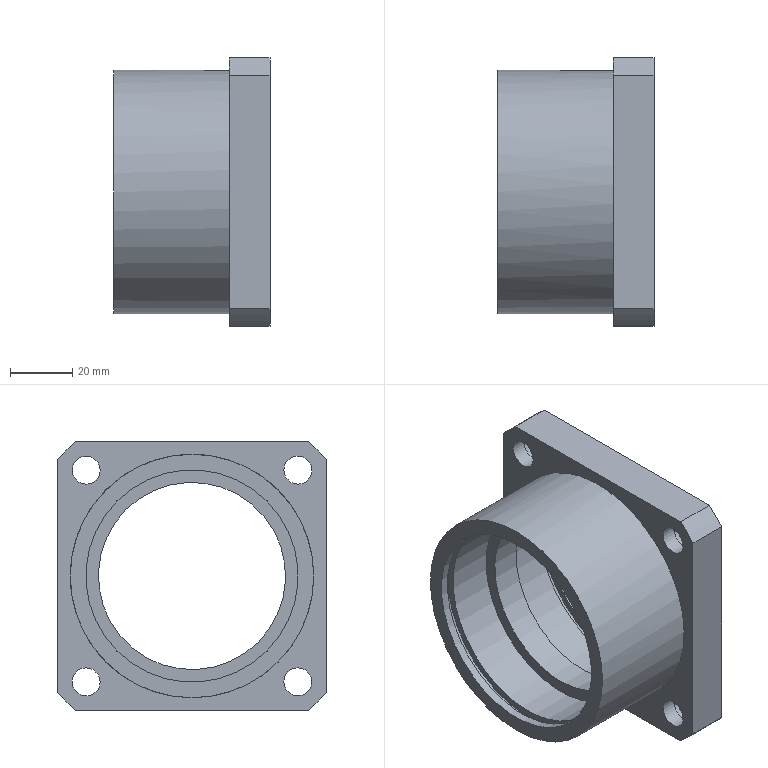Part | NX | features 1_1 2 | 1 solid | 37 faces | box 50 x 86 x 86 mm | volume 89594 mm3 | cylinder 20 | plane 17 | commonest cylinder face diameters 9 x4 14 x4 68 x4 114 x4 72.5 x2 60 x1
STEP:
#1=CARTESIAN_POINT('',(-168.3,-156.123,-789.37));
#2=VERTEX_POINT('',#1);
#3=CARTESIAN_POINT('',(-168.3,-152.941,-786.188));
#4=DIRECTION('',(1.,0.,0.));
#5=DIRECTION('',(0.,-0.7071,-0.7071));
#6=AXIS2_PLACEMENT_3D('',#3,#4,#5);
#7=CIRCLE('',#6,4.5);
#8=EDGE_CURVE('',#2,#2,#7,.T.);
#9=ORIENTED_EDGE('',*,*,#8,.F.);
#10=EDGE_LOOP('',(#9));
#11=FACE_BOUND('',#10,.T.);
#12=CARTESIAN_POINT('',(-163.4,-156.123,-789.37));
#13=VERTEX_POINT('',#12);
#14=CARTESIAN_POINT('',(-163.4,-152.941,-786.188));
#15=DIRECTION('',(-1.,0.,0.));
#16=DIRECTION('',(0.,-0.7071,-0.7071));
#17=AXIS2_PLACEMENT_3D('',#14,#15,#16);
#18=CIRCLE('',#17,4.5);
#19=EDGE_CURVE('',#13,#13,#18,.T.);
#20=ORIENTED_EDGE('',*,*,#19,.F.);
#21=EDGE_LOOP('',(#20));
#22=FACE_BOUND('',#21,.T.);
#23=CARTESIAN_POINT('',(-165.85,-152.941,-786.188));
#24=DIRECTION('',(1.,0.,0.));
#25=DIRECTION('',(0.,-0.7071,-0.7071));
#26=AXIS2_PLACEMENT_3D('',#23,#24,#25);
#27=CYLINDRICAL_SURFACE('',#26,4.5);
#28=ADVANCED_FACE('',(#11,#22),#27,.F.);
#29=ORIENTED_EDGE('',*,*,#19,.T.);
#30=EDGE_LOOP('',(#29));
#31=FACE_BOUND('',#30,.T.);
#32=CARTESIAN_POINT('',(-163.4,-147.991,-781.239));
#33=VERTEX_POINT('',#32);
#34=CARTESIAN_POINT('',(-163.4,-152.941,-786.188));
#35=DIRECTION('',(1.,0.,0.));
#36=DIRECTION('',(0.,0.7071,0.7071));
#37=AXIS2_PLACEMENT_3D('',#34,#35,#36);
#38=CIRCLE('',#37,7.);
#39=EDGE_CURVE('',#33,#33,#38,.T.);
#40=ORIENTED_EDGE('',*,*,#39,.T.);
#41=EDGE_LOOP('',(#40));
#42=FACE_BOUND('',#41,.T.);
#43=CARTESIAN_POINT('',(-163.4,-148.875,-790.254));
#44=DIRECTION('',(-1.,0.,0.));
#45=DIRECTION('',(0.,0.7071,0.7071));
#46=AXIS2_PLACEMENT_3D('',#43,#44,#45);
#47=PLANE('',#46);
#48=ADVANCED_FACE('',(#31,#42),#47,.F.);
#49=ORIENTED_EDGE('',*,*,#39,.F.);
#50=EDGE_LOOP('',(#49));
#51=FACE_BOUND('',#50,.T.);
#52=CARTESIAN_POINT('',(-155.3,-157.891,-791.138));
#53=VERTEX_POINT('',#52);
#54=CARTESIAN_POINT('',(-155.3,-152.941,-786.188));
#55=DIRECTION('',(-1.,0.,0.));
#56=DIRECTION('',(0.,-0.7071,-0.7071));
#57=AXIS2_PLACEMENT_3D('',#54,#55,#56);
#58=CIRCLE('',#57,7.);
#59=EDGE_CURVE('',#53,#53,#58,.T.);
#60=ORIENTED_EDGE('',*,*,#59,.F.);
#61=EDGE_LOOP('',(#60));
#62=FACE_BOUND('',#61,.T.);
#63=CARTESIAN_POINT('',(-159.35,-152.941,-786.188));
#64=DIRECTION('',(1.,0.,0.));
#65=DIRECTION('',(0.,-0.7071,-0.7071));
#66=AXIS2_PLACEMENT_3D('',#63,#64,#65);
#67=CYLINDRICAL_SURFACE('',#66,7.);
#68=ADVANCED_FACE('',(#51,#62),#67,.F.);
#69=CARTESIAN_POINT('',(-163.4,-88.241,-789.37));
#70=VERTEX_POINT('',#69);
#71=CARTESIAN_POINT('',(-163.4,-85.059,-786.188));
#72=DIRECTION('',(-1.,0.,0.));
#73=DIRECTION('',(0.,-0.7071,-0.7071));
#74=AXIS2_PLACEMENT_3D('',#71,#72,#73);
#75=CIRCLE('',#74,4.5);
#76=EDGE_CURVE('',#70,#70,#75,.T.);
#77=ORIENTED_EDGE('',*,*,#76,.F.);
#78=EDGE_LOOP('',(#77));
#79=FACE_BOUND('',#78,.T.);
#80=CARTESIAN_POINT('',(-168.3,-88.241,-789.37));
#81=VERTEX_POINT('',#80);
#82=CARTESIAN_POINT('',(-168.3,-85.059,-786.188));
#83=DIRECTION('',(1.,0.,0.));
#84=DIRECTION('',(0.,-0.7071,-0.7071));
#85=AXIS2_PLACEMENT_3D('',#82,#83,#84);
#86=CIRCLE('',#85,4.5);
#87=EDGE_CURVE('',#81,#81,#86,.T.);
#88=ORIENTED_EDGE('',*,*,#87,.F.);
#89=EDGE_LOOP('',(#88));
#90=FACE_BOUND('',#89,.T.);
#91=CARTESIAN_POINT('',(-165.85,-85.059,-786.188));
#92=DIRECTION('',(1.,0.,0.));
#93=DIRECTION('',(0.,-0.7071,-0.7071));
#94=AXIS2_PLACEMENT_3D('',#91,#92,#93);
#95=CYLINDRICAL_SURFACE('',#94,4.5);
#96=ADVANCED_FACE('',(#79,#90),#95,.F.);
#97=ORIENTED_EDGE('',*,*,#76,.T.);
#98=EDGE_LOOP('',(#97));
#99=FACE_BOUND('',#98,.T.);
#100=CARTESIAN_POINT('',(-163.4,-80.109,-781.239));
#101=VERTEX_POINT('',#100);
#102=CARTESIAN_POINT('',(-163.4,-85.059,-786.188));
#103=DIRECTION('',(1.,0.,0.));
#104=DIRECTION('',(0.,0.7071,0.7071));
#105=AXIS2_PLACEMENT_3D('',#102,#103,#104);
#106=CIRCLE('',#105,7.);
#107=EDGE_CURVE('',#101,#101,#106,.T.);
#108=ORIENTED_EDGE('',*,*,#107,.T.);
#109=EDGE_LOOP('',(#108));
#110=FACE_BOUND('',#109,.T.);
#111=CARTESIAN_POINT('',(-163.4,-80.993,-790.254));
#112=DIRECTION('',(-1.,0.,0.));
#113=DIRECTION('',(0.,0.7071,0.7071));
#114=AXIS2_PLACEMENT_3D('',#111,#112,#113);
#115=PLANE('',#114);
#116=ADVANCED_FACE('',(#99,#110),#115,.F.);
#117=CARTESIAN_POINT('',(-155.3,-90.009,-791.138));
#118=VERTEX_POINT('',#117);
#119=CARTESIAN_POINT('',(-155.3,-85.059,-786.188));
#120=DIRECTION('',(-1.,0.,0.));
#121=DIRECTION('',(0.,-0.7071,-0.7071));
#122=AXIS2_PLACEMENT_3D('',#119,#120,#121);
#123=CIRCLE('',#122,7.);
#124=EDGE_CURVE('',#118,#118,#123,.T.);
#125=ORIENTED_EDGE('',*,*,#124,.F.);
#126=EDGE_LOOP('',(#125));
#127=FACE_BOUND('',#126,.T.);
#128=ORIENTED_EDGE('',*,*,#107,.F.);
#129=EDGE_LOOP('',(#128));
#130=FACE_BOUND('',#129,.T.);
#131=CARTESIAN_POINT('',(-159.35,-85.059,-786.188));
#132=DIRECTION('',(1.,0.,0.));
#133=DIRECTION('',(0.,-0.7071,-0.7071));
#134=AXIS2_PLACEMENT_3D('',#131,#132,#133);
#135=CYLINDRICAL_SURFACE('',#134,7.);
#136=ADVANCED_FACE('',(#127,#130),#135,.F.);
#137=CARTESIAN_POINT('',(-168.3,-156.123,-857.253));
#138=VERTEX_POINT('',#137);
#139=CARTESIAN_POINT('',(-168.3,-152.941,-854.071));
#140=DIRECTION('',(1.,0.,0.));
#141=DIRECTION('',(0.,-0.7071,-0.7071));
#142=AXIS2_PLACEMENT_3D('',#139,#140,#141);
#143=CIRCLE('',#142,4.5);
#144=EDGE_CURVE('',#138,#138,#143,.T.);
#145=ORIENTED_EDGE('',*,*,#144,.F.);
#146=EDGE_LOOP('',(#145));
#147=FACE_BOUND('',#146,.T.);
#148=CARTESIAN_POINT('',(-163.4,-156.123,-857.253));
#149=VERTEX_POINT('',#148);
#150=CARTESIAN_POINT('',(-163.4,-152.941,-854.071));
#151=DIRECTION('',(-1.,0.,0.));
#152=DIRECTION('',(0.,-0.7071,-0.7071));
#153=AXIS2_PLACEMENT_3D('',#150,#151,#152);
#154=CIRCLE('',#153,4.5);
#155=EDGE_CURVE('',#149,#149,#154,.T.);
#156=ORIENTED_EDGE('',*,*,#155,.F.);
#157=EDGE_LOOP('',(#156));
#158=FACE_BOUND('',#157,.T.);
#159=CARTESIAN_POINT('',(-165.85,-152.941,-854.071));
#160=DIRECTION('',(1.,0.,0.));
#161=DIRECTION('',(0.,-0.7071,-0.7071));
#162=AXIS2_PLACEMENT_3D('',#159,#160,#161);
#163=CYLINDRICAL_SURFACE('',#162,4.5);
#164=ADVANCED_FACE('',(#147,#158),#163,.F.);
#165=ORIENTED_EDGE('',*,*,#155,.T.);
#166=EDGE_LOOP('',(#165));
#167=FACE_BOUND('',#166,.T.);
#168=CARTESIAN_POINT('',(-163.4,-147.991,-849.121));
#169=VERTEX_POINT('',#168);
#170=CARTESIAN_POINT('',(-163.4,-152.941,-854.071));
#171=DIRECTION('',(1.,0.,0.));
#172=DIRECTION('',(0.,0.7071,0.7071));
#173=AXIS2_PLACEMENT_3D('',#170,#171,#172);
#174=CIRCLE('',#173,7.);
#175=EDGE_CURVE('',#169,#169,#174,.T.);
#176=ORIENTED_EDGE('',*,*,#175,.T.);
#177=EDGE_LOOP('',(#176));
#178=FACE_BOUND('',#177,.T.);
#179=CARTESIAN_POINT('',(-163.4,-148.875,-858.136));
#180=DIRECTION('',(-1.,0.,0.));
#181=DIRECTION('',(0.,0.7071,0.7071));
#182=AXIS2_PLACEMENT_3D('',#179,#180,#181);
#183=PLANE('',#182);
#184=ADVANCED_FACE('',(#167,#178),#183,.F.);
#185=CARTESIAN_POINT('',(-155.3,-157.891,-859.02));
#186=VERTEX_POINT('',#185);
#187=CARTESIAN_POINT('',(-155.3,-152.941,-854.071));
#188=DIRECTION('',(-1.,0.,0.));
#189=DIRECTION('',(0.,-0.7071,-0.7071));
#190=AXIS2_PLACEMENT_3D('',#187,#188,#189);
#191=CIRCLE('',#190,7.);
#192=EDGE_CURVE('',#186,#186,#191,.T.);
#193=ORIENTED_EDGE('',*,*,#192,.F.);
#194=EDGE_LOOP('',(#193));
#195=FACE_BOUND('',#194,.T.);
#196=ORIENTED_EDGE('',*,*,#175,.F.);
#197=EDGE_LOOP('',(#196));
#198=FACE_BOUND('',#197,.T.);
#199=CARTESIAN_POINT('',(-159.35,-152.941,-854.071));
#200=DIRECTION('',(1.,0.,0.));
#201=DIRECTION('',(0.,-0.7071,-0.7071));
#202=AXIS2_PLACEMENT_3D('',#199,#200,#201);
#203=CYLINDRICAL_SURFACE('',#202,7.);
#204=ADVANCED_FACE('',(#195,#198),#203,.F.);
#205=CARTESIAN_POINT('',(-168.3,-88.241,-857.253));
#206=VERTEX_POINT('',#205);
#207=CARTESIAN_POINT('',(-168.3,-85.059,-854.071));
#208=DIRECTION('',(1.,0.,0.));
#209=DIRECTION('',(0.,-0.7071,-0.7071));
#210=AXIS2_PLACEMENT_3D('',#207,#208,#209);
#211=CIRCLE('',#210,4.5);
#212=EDGE_CURVE('',#206,#206,#211,.T.);
#213=ORIENTED_EDGE('',*,*,#212,.F.);
#214=EDGE_LOOP('',(#213));
#215=FACE_BOUND('',#214,.T.);
#216=CARTESIAN_POINT('',(-163.4,-88.241,-857.253));
#217=VERTEX_POINT('',#216);
#218=CARTESIAN_POINT('',(-163.4,-85.059,-854.071));
#219=DIRECTION('',(-1.,0.,0.));
#220=DIRECTION('',(0.,-0.7071,-0.7071));
#221=AXIS2_PLACEMENT_3D('',#218,#219,#220);
#222=CIRCLE('',#221,4.5);
#223=EDGE_CURVE('',#217,#217,#222,.T.);
#224=ORIENTED_EDGE('',*,*,#223,.F.);
#225=EDGE_LOOP('',(#224));
#226=FACE_BOUND('',#225,.T.);
#227=CARTESIAN_POINT('',(-165.85,-85.059,-854.071));
#228=DIRECTION('',(1.,0.,0.));
#229=DIRECTION('',(0.,-0.7071,-0.7071));
#230=AXIS2_PLACEMENT_3D('',#227,#228,#229);
#231=CYLINDRICAL_SURFACE('',#230,4.5);
#232=ADVANCED_FACE('',(#215,#226),#231,.F.);
#233=ORIENTED_EDGE('',*,*,#223,.T.);
#234=EDGE_LOOP('',(#233));
#235=FACE_BOUND('',#234,.T.);
#236=CARTESIAN_POINT('',(-163.4,-80.109,-849.121));
#237=VERTEX_POINT('',#236);
#238=CARTESIAN_POINT('',(-163.4,-85.059,-854.071));
#239=DIRECTION('',(1.,0.,0.));
#240=DIRECTION('',(0.,0.7071,0.7071));
#241=AXIS2_PLACEMENT_3D('',#238,#239,#240);
#242=CIRCLE('',#241,7.);
#243=EDGE_CURVE('',#237,#237,#242,.T.);
#244=ORIENTED_EDGE('',*,*,#243,.T.);
#245=EDGE_LOOP('',(#244));
#246=FACE_BOUND('',#245,.T.);
#247=CARTESIAN_POINT('',(-163.4,-80.993,-858.136));
#248=DIRECTION('',(-1.,0.,0.));
#249=DIRECTION('',(0.,0.7071,0.7071));
#250=AXIS2_PLACEMENT_3D('',#247,#248,#249);
#251=PLANE('',#250);
#252=ADVANCED_FACE('',(#235,#246),#251,.F.);
#253=ORIENTED_EDGE('',*,*,#243,.F.);
#254=EDGE_LOOP('',(#253));
#255=FACE_BOUND('',#254,.T.);
#256=CARTESIAN_POINT('',(-155.3,-90.009,-859.02));
#257=VERTEX_POINT('',#256);
#258=CARTESIAN_POINT('',(-155.3,-85.059,-854.071));
#259=DIRECTION('',(-1.,0.,0.));
#260=DIRECTION('',(0.,-0.7071,-0.7071));
#261=AXIS2_PLACEMENT_3D('',#258,#259,#260);
#262=CIRCLE('',#261,7.);
#263=EDGE_CURVE('',#257,#257,#262,.T.);
#264=ORIENTED_EDGE('',*,*,#263,.F.);
#265=EDGE_LOOP('',(#264));
#266=FACE_BOUND('',#265,.T.);
#267=CARTESIAN_POINT('',(-159.35,-85.059,-854.071));
#268=DIRECTION('',(1.,0.,0.));
#269=DIRECTION('',(0.,-0.7071,-0.7071));
#270=AXIS2_PLACEMENT_3D('',#267,#268,#269);
#271=CYLINDRICAL_SURFACE('',#270,7.);
#272=ADVANCED_FACE('',(#255,#266),#271,.F.);
#273=CARTESIAN_POINT('',(-185.1,-140.213,-841.343));
#274=VERTEX_POINT('',#273);
#275=CARTESIAN_POINT('',(-185.1,-119.,-820.129));
#276=DIRECTION('',(1.,0.,0.));
#277=DIRECTION('',(0.,-0.7071,-0.7071));
#278=AXIS2_PLACEMENT_3D('',#275,#276,#277);
#279=CIRCLE('',#278,30.);
#280=EDGE_CURVE('',#274,#274,#279,.T.);
#281=ORIENTED_EDGE('',*,*,#280,.F.);
#282=EDGE_LOOP('',(#281));
#283=FACE_BOUND('',#282,.T.);
#284=CARTESIAN_POINT('',(-175.5,-140.213,-841.343));
#285=VERTEX_POINT('',#284);
#286=CARTESIAN_POINT('',(-175.5,-119.,-820.129));
#287=DIRECTION('',(-1.,0.,0.));
#288=DIRECTION('',(0.,-0.7071,-0.7071));
#289=AXIS2_PLACEMENT_3D('',#286,#287,#288);
#290=CIRCLE('',#289,30.);
#291=EDGE_CURVE('',#285,#285,#290,.T.);
#292=ORIENTED_EDGE('',*,*,#291,.F.);
#293=EDGE_LOOP('',(#292));
#294=FACE_BOUND('',#293,.T.);
#295=CARTESIAN_POINT('',(-180.3,-119.,-820.129));
#296=DIRECTION('',(1.,0.,0.));
#297=DIRECTION('',(0.,-0.7071,-0.7071));
#298=AXIS2_PLACEMENT_3D('',#295,#296,#297);
#299=CYLINDRICAL_SURFACE('',#298,30.);
#300=ADVANCED_FACE('',(#283,#294),#299,.F.);
#301=ORIENTED_EDGE('',*,*,#291,.T.);
#302=EDGE_LOOP('',(#301));
#303=FACE_BOUND('',#302,.T.);
#304=CARTESIAN_POINT('',(-175.5,-94.958,-796.088));
#305=VERTEX_POINT('',#304);
#306=CARTESIAN_POINT('',(-175.5,-119.,-820.129));
#307=DIRECTION('',(1.,0.,0.));
#308=DIRECTION('',(0.,0.7071,0.7071));
#309=AXIS2_PLACEMENT_3D('',#306,#307,#308);
#310=CIRCLE('',#309,34.);
#311=EDGE_CURVE('',#305,#305,#310,.T.);
#312=ORIENTED_EDGE('',*,*,#311,.T.);
#313=EDGE_LOOP('',(#312));
#314=FACE_BOUND('',#313,.T.);
#315=CARTESIAN_POINT('',(-175.5,-96.373,-842.757));
#316=DIRECTION('',(1.,0.,0.));
#317=DIRECTION('',(0.,-0.7071,-0.7071));
#318=AXIS2_PLACEMENT_3D('',#315,#316,#317);
#319=PLANE('',#318);
#320=ADVANCED_FACE('',(#303,#314),#319,.T.);
#321=ORIENTED_EDGE('',*,*,#311,.F.);
#322=EDGE_LOOP('',(#321));
#323=FACE_BOUND('',#322,.T.);
#324=CARTESIAN_POINT('',(-160.5,-143.042,-844.171));
#325=VERTEX_POINT('',#324);
#326=CARTESIAN_POINT('',(-160.5,-119.,-820.129));
#327=DIRECTION('',(-1.,0.,0.));
#328=DIRECTION('',(0.,-0.7071,-0.7071));
#329=AXIS2_PLACEMENT_3D('',#326,#327,#328);
#330=CIRCLE('',#329,34.);
#331=EDGE_CURVE('',#325,#325,#330,.T.);
#332=ORIENTED_EDGE('',*,*,#331,.F.);
#333=EDGE_LOOP('',(#332));
#334=FACE_BOUND('',#333,.T.);
#335=CARTESIAN_POINT('',(-168.,-119.,-820.129));
#336=DIRECTION('',(1.,0.,0.));
#337=DIRECTION('',(0.,-0.7071,-0.7071));
#338=AXIS2_PLACEMENT_3D('',#335,#336,#337);
#339=CYLINDRICAL_SURFACE('',#338,34.);
#340=ADVANCED_FACE('',(#323,#334),#339,.F.);
#341=ORIENTED_EDGE('',*,*,#331,.T.);
#342=EDGE_LOOP('',(#341));
#343=FACE_BOUND('',#342,.T.);
#344=CARTESIAN_POINT('',(-160.5,-93.367,-794.497));
#345=VERTEX_POINT('',#344);
#346=CARTESIAN_POINT('',(-160.5,-119.,-820.129));
#347=DIRECTION('',(1.,0.,0.));
#348=DIRECTION('',(0.,0.7071,0.7071));
#349=AXIS2_PLACEMENT_3D('',#346,#347,#348);
#350=CIRCLE('',#349,36.25);
#351=EDGE_CURVE('',#345,#345,#350,.T.);
#352=ORIENTED_EDGE('',*,*,#351,.T.);
#353=EDGE_LOOP('',(#352));
#354=FACE_BOUND('',#353,.T.);
#355=CARTESIAN_POINT('',(-160.5,-94.163,-844.967));
#356=DIRECTION('',(1.,0.,0.));
#357=DIRECTION('',(0.,0.7071,-0.7071));
#358=AXIS2_PLACEMENT_3D('',#355,#356,#357);
#359=PLANE('',#358);
#360=ADVANCED_FACE('',(#343,#354),#359,.T.);
#361=ORIENTED_EDGE('',*,*,#351,.F.);
#362=EDGE_LOOP('',(#361));
#363=FACE_BOUND('',#362,.T.);
#364=CARTESIAN_POINT('',(-158.,-144.633,-845.762));
#365=VERTEX_POINT('',#364);
#366=CARTESIAN_POINT('',(-158.,-119.,-820.129));
#367=DIRECTION('',(-1.,0.,0.));
#368=DIRECTION('',(0.,-0.7071,-0.7071));
#369=AXIS2_PLACEMENT_3D('',#366,#367,#368);
#370=CIRCLE('',#369,36.25);
#371=EDGE_CURVE('',#365,#365,#370,.T.);
#372=ORIENTED_EDGE('',*,*,#371,.F.);
#373=EDGE_LOOP('',(#372));
#374=FACE_BOUND('',#373,.T.);
#375=CARTESIAN_POINT('',(-159.25,-119.,-820.129));
#376=DIRECTION('',(1.,0.,0.));
#377=DIRECTION('',(0.,-0.7071,-0.7071));
#378=AXIS2_PLACEMENT_3D('',#375,#376,#377);
#379=CYLINDRICAL_SURFACE('',#378,36.25);
#380=ADVANCED_FACE('',(#363,#374),#379,.F.);
#381=CARTESIAN_POINT('',(-158.,-94.958,-796.088));
#382=VERTEX_POINT('',#381);
#383=CARTESIAN_POINT('',(-158.,-119.,-820.129));
#384=DIRECTION('',(1.,0.,0.));
#385=DIRECTION('',(0.,0.7071,0.7071));
#386=AXIS2_PLACEMENT_3D('',#383,#384,#385);
#387=CIRCLE('',#386,34.);
#388=EDGE_CURVE('',#382,#382,#387,.T.);
#389=ORIENTED_EDGE('',*,*,#388,.T.);
#390=EDGE_LOOP('',(#389));
#391=FACE_BOUND('',#390,.T.);
#392=ORIENTED_EDGE('',*,*,#371,.T.);
#393=EDGE_LOOP('',(#392));
#394=FACE_BOUND('',#393,.T.);
#395=CARTESIAN_POINT('',(-158.,-94.163,-844.967));
#396=DIRECTION('',(-1.,0.,0.));
#397=DIRECTION('',(0.,0.7071,0.7071));
#398=AXIS2_PLACEMENT_3D('',#395,#396,#397);
#399=PLANE('',#398);
#400=ADVANCED_FACE('',(#391,#394),#399,.T.);
#401=CARTESIAN_POINT('',(-155.3,-143.042,-844.171));
#402=VERTEX_POINT('',#401);
#403=CARTESIAN_POINT('',(-155.3,-119.,-820.129));
#404=DIRECTION('',(-1.,0.,0.));
#405=DIRECTION('',(0.,-0.7071,-0.7071));
#406=AXIS2_PLACEMENT_3D('',#403,#404,#405);
#407=CIRCLE('',#406,34.);
#408=EDGE_CURVE('',#402,#402,#407,.T.);
#409=ORIENTED_EDGE('',*,*,#408,.F.);
#410=EDGE_LOOP('',(#409));
#411=FACE_BOUND('',#410,.T.);
#412=ORIENTED_EDGE('',*,*,#388,.F.);
#413=EDGE_LOOP('',(#412));
#414=FACE_BOUND('',#413,.T.);
#415=CARTESIAN_POINT('',(-156.65,-119.,-820.129));
#416=DIRECTION('',(1.,0.,0.));
#417=DIRECTION('',(0.,-0.7071,-0.7071));
#418=AXIS2_PLACEMENT_3D('',#415,#416,#417);
#419=CYLINDRICAL_SURFACE('',#418,34.);
#420=ADVANCED_FACE('',(#411,#414),#419,.F.);
#421=CARTESIAN_POINT('',(-168.3,-81.583,-777.129));
#422=VERTEX_POINT('',#421);
#423=CARTESIAN_POINT('',(-168.3,-76.,-782.713));
#424=VERTEX_POINT('',#423);
#425=CARTESIAN_POINT('',(-168.3,-119.,-820.129));
#426=DIRECTION('',(-1.,0.,0.));
#427=DIRECTION('',(0.,0.7071,0.7071));
#428=AXIS2_PLACEMENT_3D('',#425,#426,#427);
#429=CIRCLE('',#428,57.);
#430=EDGE_CURVE('',#422,#424,#429,.T.);
#431=ORIENTED_EDGE('',*,*,#430,.F.);
#432=CARTESIAN_POINT('',(-155.3,-81.583,-777.129));
#433=VERTEX_POINT('',#432);
#434=CARTESIAN_POINT('',(-168.3,-81.583,-777.129));
#435=DIRECTION('',(1.,0.,0.));
#436=VECTOR('',#435,1000.);
#437=LINE('',#434,#436);
#438=EDGE_CURVE('',#422,#433,#437,.T.);
#439=ORIENTED_EDGE('',*,*,#438,.T.);
#440=CARTESIAN_POINT('',(-155.3,-76.,-782.713));
#441=VERTEX_POINT('',#440);
#442=CARTESIAN_POINT('',(-155.3,-119.,-820.129));
#443=DIRECTION('',(1.,0.,0.));
#444=DIRECTION('',(0.,0.7071,0.7071));
#445=AXIS2_PLACEMENT_3D('',#442,#443,#444);
#446=CIRCLE('',#445,57.);
#447=EDGE_CURVE('',#441,#433,#446,.T.);
#448=ORIENTED_EDGE('',*,*,#447,.F.);
#449=CARTESIAN_POINT('',(-155.3,-76.,-782.713));
#450=DIRECTION('',(-1.,0.,0.));
#451=VECTOR('',#450,1000.);
#452=LINE('',#449,#451);
#453=EDGE_CURVE('',#441,#424,#452,.T.);
#454=ORIENTED_EDGE('',*,*,#453,.T.);
#455=EDGE_LOOP('',(#431,#439,#448,#454));
#456=FACE_BOUND('',#455,.T.);
#457=CARTESIAN_POINT('',(-161.8,-119.,-820.129));
#458=DIRECTION('',(1.,0.,0.));
#459=DIRECTION('',(0.,-0.7071,-0.7071));
#460=AXIS2_PLACEMENT_3D('',#457,#458,#459);
#461=CYLINDRICAL_SURFACE('',#460,57.);
#462=ADVANCED_FACE('',(#456),#461,.T.);
#463=ORIENTED_EDGE('',*,*,#438,.F.);
#464=CARTESIAN_POINT('',(-168.3,-156.417,-777.129));
#465=VERTEX_POINT('',#464);
#466=CARTESIAN_POINT('',(-168.3,-156.417,-777.129));
#467=DIRECTION('',(0.,1.,0.));
#468=VECTOR('',#467,1000.);
#469=LINE('',#466,#468);
#470=EDGE_CURVE('',#465,#422,#469,.T.);
#471=ORIENTED_EDGE('',*,*,#470,.F.);
#472=CARTESIAN_POINT('',(-155.3,-156.417,-777.129));
#473=VERTEX_POINT('',#472);
#474=CARTESIAN_POINT('',(-155.3,-156.417,-777.129));
#475=DIRECTION('',(-1.,0.,0.));
#476=VECTOR('',#475,1000.);
#477=LINE('',#474,#476);
#478=EDGE_CURVE('',#473,#465,#477,.T.);
#479=ORIENTED_EDGE('',*,*,#478,.F.);
#480=CARTESIAN_POINT('',(-155.3,-81.583,-777.129));
#481=DIRECTION('',(0.,-1.,0.));
#482=VECTOR('',#481,1000.);
#483=LINE('',#480,#482);
#484=EDGE_CURVE('',#433,#473,#483,.T.);
#485=ORIENTED_EDGE('',*,*,#484,.F.);
#486=EDGE_LOOP('',(#463,#471,#479,#485));
#487=FACE_BOUND('',#486,.T.);
#488=CARTESIAN_POINT('',(-155.3,-162.,-777.129));
#489=DIRECTION('',(0.,0.,-1.));
#490=DIRECTION('',(0.,1.,0.));
#491=AXIS2_PLACEMENT_3D('',#488,#489,#490);
#492=PLANE('',#491);
#493=ADVANCED_FACE('',(#487),#492,.F.);
#494=CARTESIAN_POINT('',(-168.3,-162.,-782.713));
#495=VERTEX_POINT('',#494);
#496=CARTESIAN_POINT('',(-168.3,-119.,-820.129));
#497=DIRECTION('',(-1.,0.,0.));
#498=DIRECTION('',(0.,-0.7544,0.6564));
#499=AXIS2_PLACEMENT_3D('',#496,#497,#498);
#500=CIRCLE('',#499,57.);
#501=EDGE_CURVE('',#495,#465,#500,.T.);
#502=ORIENTED_EDGE('',*,*,#501,.F.);
#503=CARTESIAN_POINT('',(-155.3,-162.,-782.713));
#504=VERTEX_POINT('',#503);
#505=CARTESIAN_POINT('',(-168.3,-162.,-782.713));
#506=DIRECTION('',(1.,0.,0.));
#507=VECTOR('',#506,1000.);
#508=LINE('',#505,#507);
#509=EDGE_CURVE('',#495,#504,#508,.T.);
#510=ORIENTED_EDGE('',*,*,#509,.T.);
#511=CARTESIAN_POINT('',(-155.3,-119.,-820.129));
#512=DIRECTION('',(1.,0.,0.));
#513=DIRECTION('',(0.,-0.6564,0.7544));
#514=AXIS2_PLACEMENT_3D('',#511,#512,#513);
#515=CIRCLE('',#514,57.);
#516=EDGE_CURVE('',#473,#504,#515,.T.);
#517=ORIENTED_EDGE('',*,*,#516,.F.);
#518=ORIENTED_EDGE('',*,*,#478,.T.);
#519=EDGE_LOOP('',(#502,#510,#517,#518));
#520=FACE_BOUND('',#519,.T.);
#521=CARTESIAN_POINT('',(-161.8,-119.,-820.129));
#522=DIRECTION('',(1.,0.,0.));
#523=DIRECTION('',(0.,-0.7071,-0.7071));
#524=AXIS2_PLACEMENT_3D('',#521,#522,#523);
#525=CYLINDRICAL_SURFACE('',#524,57.);
#526=ADVANCED_FACE('',(#520),#525,.T.);
#527=CARTESIAN_POINT('',(-168.3,-76.,-857.546));
#528=VERTEX_POINT('',#527);
#529=CARTESIAN_POINT('',(-168.3,-81.583,-863.129));
#530=VERTEX_POINT('',#529);
#531=CARTESIAN_POINT('',(-168.3,-119.,-820.129));
#532=DIRECTION('',(-1.,0.,0.));
#533=DIRECTION('',(0.,0.7544,-0.6564));
#534=AXIS2_PLACEMENT_3D('',#531,#532,#533);
#535=CIRCLE('',#534,57.);
#536=EDGE_CURVE('',#528,#530,#535,.T.);
#537=ORIENTED_EDGE('',*,*,#536,.F.);
#538=CARTESIAN_POINT('',(-155.3,-76.,-857.546));
#539=VERTEX_POINT('',#538);
#540=CARTESIAN_POINT('',(-168.3,-76.,-857.546));
#541=DIRECTION('',(1.,0.,0.));
#542=VECTOR('',#541,1000.);
#543=LINE('',#540,#542);
#544=EDGE_CURVE('',#528,#539,#543,.T.);
#545=ORIENTED_EDGE('',*,*,#544,.T.);
#546=CARTESIAN_POINT('',(-155.3,-81.583,-863.129));
#547=VERTEX_POINT('',#546);
#548=CARTESIAN_POINT('',(-155.3,-119.,-820.129));
#549=DIRECTION('',(1.,0.,0.));
#550=DIRECTION('',(0.,0.6564,-0.7544));
#551=AXIS2_PLACEMENT_3D('',#548,#549,#550);
#552=CIRCLE('',#551,57.);
#553=EDGE_CURVE('',#547,#539,#552,.T.);
#554=ORIENTED_EDGE('',*,*,#553,.F.);
#555=CARTESIAN_POINT('',(-155.3,-81.583,-863.129));
#556=DIRECTION('',(-1.,0.,0.));
#557=VECTOR('',#556,1000.);
#558=LINE('',#555,#557);
#559=EDGE_CURVE('',#547,#530,#558,.T.);
#560=ORIENTED_EDGE('',*,*,#559,.T.);
#561=EDGE_LOOP('',(#537,#545,#554,#560));
#562=FACE_BOUND('',#561,.T.);
#563=CARTESIAN_POINT('',(-161.8,-119.,-820.129));
#564=DIRECTION('',(1.,0.,0.));
#565=DIRECTION('',(0.,-0.7071,-0.7071));
#566=AXIS2_PLACEMENT_3D('',#563,#564,#565);
#567=CYLINDRICAL_SURFACE('',#566,57.);
#568=ADVANCED_FACE('',(#562),#567,.T.);
#569=CARTESIAN_POINT('',(-168.3,-156.417,-863.129));
#570=VERTEX_POINT('',#569);
#571=CARTESIAN_POINT('',(-155.3,-156.417,-863.129));
#572=VERTEX_POINT('',#571);
#573=CARTESIAN_POINT('',(-168.3,-156.417,-863.129));
#574=DIRECTION('',(1.,0.,0.));
#575=VECTOR('',#574,1000.);
#576=LINE('',#573,#575);
#577=EDGE_CURVE('',#570,#572,#576,.T.);
#578=ORIENTED_EDGE('',*,*,#577,.F.);
#579=CARTESIAN_POINT('',(-168.3,-81.583,-863.129));
#580=DIRECTION('',(0.,-1.,0.));
#581=VECTOR('',#580,1000.);
#582=LINE('',#579,#581);
#583=EDGE_CURVE('',#530,#570,#582,.T.);
#584=ORIENTED_EDGE('',*,*,#583,.F.);
#585=ORIENTED_EDGE('',*,*,#559,.F.);
#586=CARTESIAN_POINT('',(-155.3,-156.417,-863.129));
#587=DIRECTION('',(0.,1.,0.));
#588=VECTOR('',#587,1000.);
#589=LINE('',#586,#588);
#590=EDGE_CURVE('',#572,#547,#589,.T.);
#591=ORIENTED_EDGE('',*,*,#590,.F.);
#592=EDGE_LOOP('',(#578,#584,#585,#591));
#593=FACE_BOUND('',#592,.T.);
#594=CARTESIAN_POINT('',(-155.3,-76.,-863.129));
#595=DIRECTION('',(0.,0.,1.));
#596=DIRECTION('',(0.,-1.,0.));
#597=AXIS2_PLACEMENT_3D('',#594,#595,#596);
#598=PLANE('',#597);
#599=ADVANCED_FACE('',(#593),#598,.F.);
#600=CARTESIAN_POINT('',(-168.3,-162.,-857.546));
#601=VERTEX_POINT('',#600);
#602=CARTESIAN_POINT('',(-168.3,-119.,-820.129));
#603=DIRECTION('',(-1.,0.,0.));
#604=DIRECTION('',(0.,-0.7071,-0.7071));
#605=AXIS2_PLACEMENT_3D('',#602,#603,#604);
#606=CIRCLE('',#605,57.);
#607=EDGE_CURVE('',#570,#601,#606,.T.);
#608=ORIENTED_EDGE('',*,*,#607,.F.);
#609=ORIENTED_EDGE('',*,*,#577,.T.);
#610=CARTESIAN_POINT('',(-155.3,-162.,-857.546));
#611=VERTEX_POINT('',#610);
#612=CARTESIAN_POINT('',(-155.3,-119.,-820.129));
#613=DIRECTION('',(1.,0.,0.));
#614=DIRECTION('',(0.,-0.7071,-0.7071));
#615=AXIS2_PLACEMENT_3D('',#612,#613,#614);
#616=CIRCLE('',#615,57.);
#617=EDGE_CURVE('',#611,#572,#616,.T.);
#618=ORIENTED_EDGE('',*,*,#617,.F.);
#619=CARTESIAN_POINT('',(-155.3,-162.,-857.546));
#620=DIRECTION('',(-1.,0.,0.));
#621=VECTOR('',#620,1000.);
#622=LINE('',#619,#621);
#623=EDGE_CURVE('',#611,#601,#622,.T.);
#624=ORIENTED_EDGE('',*,*,#623,.T.);
#625=EDGE_LOOP('',(#608,#609,#618,#624));
#626=FACE_BOUND('',#625,.T.);
#627=CARTESIAN_POINT('',(-161.8,-119.,-820.129));
#628=DIRECTION('',(1.,0.,0.));
#629=DIRECTION('',(0.,-0.7071,-0.7071));
#630=AXIS2_PLACEMENT_3D('',#627,#628,#629);
#631=CYLINDRICAL_SURFACE('',#630,57.);
#632=ADVANCED_FACE('',(#626),#631,.T.);
#633=ORIENTED_EDGE('',*,*,#509,.F.);
#634=CARTESIAN_POINT('',(-168.3,-162.,-857.546));
#635=DIRECTION('',(0.,0.,1.));
#636=VECTOR('',#635,1000.);
#637=LINE('',#634,#636);
#638=EDGE_CURVE('',#601,#495,#637,.T.);
#639=ORIENTED_EDGE('',*,*,#638,.F.);
#640=ORIENTED_EDGE('',*,*,#623,.F.);
#641=CARTESIAN_POINT('',(-155.3,-162.,-782.713));
#642=DIRECTION('',(0.,0.,-1.));
#643=VECTOR('',#642,1000.);
#644=LINE('',#641,#643);
#645=EDGE_CURVE('',#504,#611,#644,.T.);
#646=ORIENTED_EDGE('',*,*,#645,.F.);
#647=EDGE_LOOP('',(#633,#639,#640,#646));
#648=FACE_BOUND('',#647,.T.);
#649=CARTESIAN_POINT('',(-155.3,-162.,-863.129));
#650=DIRECTION('',(0.,1.,0.));
#651=DIRECTION('',(0.,0.,1.));
#652=AXIS2_PLACEMENT_3D('',#649,#650,#651);
#653=PLANE('',#652);
#654=ADVANCED_FACE('',(#648),#653,.F.);
#655=ORIENTED_EDGE('',*,*,#59,.T.);
#656=EDGE_LOOP('',(#655));
#657=FACE_BOUND('',#656,.T.);
#658=ORIENTED_EDGE('',*,*,#124,.T.);
#659=EDGE_LOOP('',(#658));
#660=FACE_BOUND('',#659,.T.);
#661=ORIENTED_EDGE('',*,*,#192,.T.);
#662=EDGE_LOOP('',(#661));
#663=FACE_BOUND('',#662,.T.);
#664=ORIENTED_EDGE('',*,*,#263,.T.);
#665=EDGE_LOOP('',(#664));
#666=FACE_BOUND('',#665,.T.);
#667=ORIENTED_EDGE('',*,*,#408,.T.);
#668=EDGE_LOOP('',(#667));
#669=FACE_BOUND('',#668,.T.);
#670=ORIENTED_EDGE('',*,*,#645,.T.);
#671=ORIENTED_EDGE('',*,*,#617,.T.);
#672=ORIENTED_EDGE('',*,*,#590,.T.);
#673=ORIENTED_EDGE('',*,*,#553,.T.);
#674=CARTESIAN_POINT('',(-155.3,-76.,-857.546));
#675=DIRECTION('',(0.,0.,1.));
#676=VECTOR('',#675,1000.);
#677=LINE('',#674,#676);
#678=EDGE_CURVE('',#539,#441,#677,.T.);
#679=ORIENTED_EDGE('',*,*,#678,.T.);
#680=ORIENTED_EDGE('',*,*,#447,.T.);
#681=ORIENTED_EDGE('',*,*,#484,.T.);
#682=ORIENTED_EDGE('',*,*,#516,.T.);
#683=EDGE_LOOP('',(#670,#671,#672,#673,#679,#680,#681,#682));
#684=FACE_BOUND('',#683,.T.);
#685=CARTESIAN_POINT('',(-155.3,-86.827,-852.303));
#686=DIRECTION('',(1.,0.,0.));
#687=DIRECTION('',(0.,-0.7071,-0.7071));
#688=AXIS2_PLACEMENT_3D('',#685,#686,#687);
#689=PLANE('',#688);
#690=ADVANCED_FACE('',(#657,#660,#663,#666,#669,#684),#689,.T.);
#691=ORIENTED_EDGE('',*,*,#544,.F.);
#692=CARTESIAN_POINT('',(-168.3,-76.,-782.713));
#693=DIRECTION('',(0.,0.,-1.));
#694=VECTOR('',#693,1000.);
#695=LINE('',#692,#694);
#696=EDGE_CURVE('',#424,#528,#695,.T.);
#697=ORIENTED_EDGE('',*,*,#696,.F.);
#698=ORIENTED_EDGE('',*,*,#453,.F.);
#699=ORIENTED_EDGE('',*,*,#678,.F.);
#700=EDGE_LOOP('',(#691,#697,#698,#699));
#701=FACE_BOUND('',#700,.T.);
#702=CARTESIAN_POINT('',(-155.3,-76.,-777.129));
#703=DIRECTION('',(0.,-1.,0.));
#704=DIRECTION('',(0.,0.,-1.));
#705=AXIS2_PLACEMENT_3D('',#702,#703,#704);
#706=PLANE('',#705);
#707=ADVANCED_FACE('',(#701),#706,.F.);
#708=ORIENTED_EDGE('',*,*,#8,.T.);
#709=EDGE_LOOP('',(#708));
#710=FACE_BOUND('',#709,.T.);
#711=ORIENTED_EDGE('',*,*,#87,.T.);
#712=EDGE_LOOP('',(#711));
#713=FACE_BOUND('',#712,.T.);
#714=ORIENTED_EDGE('',*,*,#144,.T.);
#715=EDGE_LOOP('',(#714));
#716=FACE_BOUND('',#715,.T.);
#717=ORIENTED_EDGE('',*,*,#212,.T.);
#718=EDGE_LOOP('',(#717));
#719=FACE_BOUND('',#718,.T.);
#720=CARTESIAN_POINT('',(-168.3,-146.577,-847.707));
#721=VERTEX_POINT('',#720);
#722=CARTESIAN_POINT('',(-168.3,-119.,-820.129));
#723=DIRECTION('',(1.,0.,0.));
#724=DIRECTION('',(0.,-0.7071,-0.7071));
#725=AXIS2_PLACEMENT_3D('',#722,#723,#724);
#726=CIRCLE('',#725,39.);
#727=EDGE_CURVE('',#721,#721,#726,.T.);
#728=ORIENTED_EDGE('',*,*,#727,.T.);
#729=EDGE_LOOP('',(#728));
#730=FACE_BOUND('',#729,.T.);
#731=ORIENTED_EDGE('',*,*,#536,.T.);
#732=ORIENTED_EDGE('',*,*,#583,.T.);
#733=ORIENTED_EDGE('',*,*,#607,.T.);
#734=ORIENTED_EDGE('',*,*,#638,.T.);
#735=ORIENTED_EDGE('',*,*,#501,.T.);
#736=ORIENTED_EDGE('',*,*,#470,.T.);
#737=ORIENTED_EDGE('',*,*,#430,.T.);
#738=ORIENTED_EDGE('',*,*,#696,.T.);
#739=EDGE_LOOP('',(#731,#732,#733,#734,#735,#736,#737,#738));
#740=FACE_BOUND('',#739,.T.);
#741=CARTESIAN_POINT('',(-168.3,-85.059,-854.071));
#742=DIRECTION('',(-1.,0.,0.));
#743=DIRECTION('',(0.,0.7071,0.7071));
#744=AXIS2_PLACEMENT_3D('',#741,#742,#743);
#745=PLANE('',#744);
#746=ADVANCED_FACE('',(#710,#713,#716,#719,#730,#740),#745,.T.);
#747=ORIENTED_EDGE('',*,*,#727,.F.);
#748=EDGE_LOOP('',(#747));
#749=FACE_BOUND('',#748,.T.);
#750=CARTESIAN_POINT('',(-205.3,-91.423,-792.552));
#751=VERTEX_POINT('',#750);
#752=CARTESIAN_POINT('',(-205.3,-119.,-820.129));
#753=DIRECTION('',(-1.,0.,0.));
#754=DIRECTION('',(0.,0.7071,0.7071));
#755=AXIS2_PLACEMENT_3D('',#752,#753,#754);
#756=CIRCLE('',#755,39.);
#757=EDGE_CURVE('',#751,#751,#756,.T.);
#758=ORIENTED_EDGE('',*,*,#757,.F.);
#759=EDGE_LOOP('',(#758));
#760=FACE_BOUND('',#759,.T.);
#761=CARTESIAN_POINT('',(-186.8,-119.,-820.129));
#762=DIRECTION('',(1.,0.,0.));
#763=DIRECTION('',(0.,-0.7071,-0.7071));
#764=AXIS2_PLACEMENT_3D('',#761,#762,#763);
#765=CYLINDRICAL_SURFACE('',#764,39.);
#766=ADVANCED_FACE('',(#749,#760),#765,.T.);
#767=CARTESIAN_POINT('',(-205.3,-94.958,-796.088));
#768=VERTEX_POINT('',#767);
#769=CARTESIAN_POINT('',(-205.3,-119.,-820.129));
#770=DIRECTION('',(1.,0.,0.));
#771=DIRECTION('',(0.,0.7071,0.7071));
#772=AXIS2_PLACEMENT_3D('',#769,#770,#771);
#773=CIRCLE('',#772,34.);
#774=EDGE_CURVE('',#768,#768,#773,.T.);
#775=ORIENTED_EDGE('',*,*,#774,.T.);
#776=EDGE_LOOP('',(#775));
#777=FACE_BOUND('',#776,.T.);
#778=ORIENTED_EDGE('',*,*,#757,.T.);
#779=EDGE_LOOP('',(#778));
#780=FACE_BOUND('',#779,.T.);
#781=CARTESIAN_POINT('',(-205.3,-93.191,-845.939));
#782=DIRECTION('',(-1.,0.,0.));
#783=DIRECTION('',(0.,0.7071,0.7071));
#784=AXIS2_PLACEMENT_3D('',#781,#782,#783);
#785=PLANE('',#784);
#786=ADVANCED_FACE('',(#777,#780),#785,.T.);
#787=CARTESIAN_POINT('',(-202.6,-143.042,-844.171));
#788=VERTEX_POINT('',#787);
#789=CARTESIAN_POINT('',(-202.6,-119.,-820.129));
#790=DIRECTION('',(-1.,0.,0.));
#791=DIRECTION('',(0.,-0.7071,-0.7071));
#792=AXIS2_PLACEMENT_3D('',#789,#790,#791);
#793=CIRCLE('',#792,34.);
#794=EDGE_CURVE('',#788,#788,#793,.T.);
#795=ORIENTED_EDGE('',*,*,#794,.F.);
#796=EDGE_LOOP('',(#795));
#797=FACE_BOUND('',#796,.T.);
#798=ORIENTED_EDGE('',*,*,#774,.F.);
#799=EDGE_LOOP('',(#798));
#800=FACE_BOUND('',#799,.T.);
#801=CARTESIAN_POINT('',(-203.95,-119.,-820.129));
#802=DIRECTION('',(1.,0.,0.));
#803=DIRECTION('',(0.,-0.7071,-0.7071));
#804=AXIS2_PLACEMENT_3D('',#801,#802,#803);
#805=CYLINDRICAL_SURFACE('',#804,34.);
#806=ADVANCED_FACE('',(#797,#800),#805,.F.);
#807=ORIENTED_EDGE('',*,*,#794,.T.);
#808=EDGE_LOOP('',(#807));
#809=FACE_BOUND('',#808,.T.);
#810=CARTESIAN_POINT('',(-202.6,-93.367,-794.497));
#811=VERTEX_POINT('',#810);
#812=CARTESIAN_POINT('',(-202.6,-119.,-820.129));
#813=DIRECTION('',(1.,0.,0.));
#814=DIRECTION('',(0.,0.7071,0.7071));
#815=AXIS2_PLACEMENT_3D('',#812,#813,#814);
#816=CIRCLE('',#815,36.25);
#817=EDGE_CURVE('',#811,#811,#816,.T.);
#818=ORIENTED_EDGE('',*,*,#817,.T.);
#819=EDGE_LOOP('',(#818));
#820=FACE_BOUND('',#819,.T.);
#821=CARTESIAN_POINT('',(-202.6,-94.163,-844.967));
#822=DIRECTION('',(1.,0.,0.));
#823=DIRECTION('',(0.,-0.7071,-0.7071));
#824=AXIS2_PLACEMENT_3D('',#821,#822,#823);
#825=PLANE('',#824);
#826=ADVANCED_FACE('',(#809,#820),#825,.T.);
#827=CARTESIAN_POINT('',(-200.1,-144.633,-845.762));
#828=VERTEX_POINT('',#827);
#829=CARTESIAN_POINT('',(-200.1,-119.,-820.129));
#830=DIRECTION('',(-1.,0.,0.));
#831=DIRECTION('',(0.,-0.7071,-0.7071));
#832=AXIS2_PLACEMENT_3D('',#829,#830,#831);
#833=CIRCLE('',#832,36.25);
#834=EDGE_CURVE('',#828,#828,#833,.T.);
#835=ORIENTED_EDGE('',*,*,#834,.F.);
#836=EDGE_LOOP('',(#835));
#837=FACE_BOUND('',#836,.T.);
#838=ORIENTED_EDGE('',*,*,#817,.F.);
#839=EDGE_LOOP('',(#838));
#840=FACE_BOUND('',#839,.T.);
#841=CARTESIAN_POINT('',(-201.35,-119.,-820.129));
#842=DIRECTION('',(1.,0.,0.));
#843=DIRECTION('',(0.,-0.7071,-0.7071));
#844=AXIS2_PLACEMENT_3D('',#841,#842,#843);
#845=CYLINDRICAL_SURFACE('',#844,36.25);
#846=ADVANCED_FACE('',(#837,#840),#845,.F.);
#847=CARTESIAN_POINT('',(-200.1,-94.958,-796.088));
#848=VERTEX_POINT('',#847);
#849=CARTESIAN_POINT('',(-200.1,-119.,-820.129));
#850=DIRECTION('',(1.,0.,0.));
#851=DIRECTION('',(0.,0.7071,0.7071));
#852=AXIS2_PLACEMENT_3D('',#849,#850,#851);
#853=CIRCLE('',#852,34.);
#854=EDGE_CURVE('',#848,#848,#853,.T.);
#855=ORIENTED_EDGE('',*,*,#854,.T.);
#856=EDGE_LOOP('',(#855));
#857=FACE_BOUND('',#856,.T.);
#858=ORIENTED_EDGE('',*,*,#834,.T.);
#859=EDGE_LOOP('',(#858));
#860=FACE_BOUND('',#859,.T.);
#861=CARTESIAN_POINT('',(-200.1,-94.163,-844.967));
#862=DIRECTION('',(-1.,0.,0.));
#863=DIRECTION('',(0.,0.7071,0.7071));
#864=AXIS2_PLACEMENT_3D('',#861,#862,#863);
#865=PLANE('',#864);
#866=ADVANCED_FACE('',(#857,#860),#865,.T.);
#867=ORIENTED_EDGE('',*,*,#854,.F.);
#868=EDGE_LOOP('',(#867));
#869=FACE_BOUND('',#868,.T.);
#870=CARTESIAN_POINT('',(-185.1,-143.042,-844.171));
#871=VERTEX_POINT('',#870);
#872=CARTESIAN_POINT('',(-185.1,-119.,-820.129));
#873=DIRECTION('',(-1.,0.,0.));
#874=DIRECTION('',(0.,-0.7071,-0.7071));
#875=AXIS2_PLACEMENT_3D('',#872,#873,#874);
#876=CIRCLE('',#875,34.);
#877=EDGE_CURVE('',#871,#871,#876,.T.);
#878=ORIENTED_EDGE('',*,*,#877,.F.);
#879=EDGE_LOOP('',(#878));
#880=FACE_BOUND('',#879,.T.);
#881=CARTESIAN_POINT('',(-192.6,-119.,-820.129));
#882=DIRECTION('',(1.,0.,0.));
#883=DIRECTION('',(0.,-0.7071,-0.7071));
#884=AXIS2_PLACEMENT_3D('',#881,#882,#883);
#885=CYLINDRICAL_SURFACE('',#884,34.);
#886=ADVANCED_FACE('',(#869,#880),#885,.F.);
#887=ORIENTED_EDGE('',*,*,#280,.T.);
#888=EDGE_LOOP('',(#887));
#889=FACE_BOUND('',#888,.T.);
#890=ORIENTED_EDGE('',*,*,#877,.T.);
#891=EDGE_LOOP('',(#890));
#892=FACE_BOUND('',#891,.T.);
#893=CARTESIAN_POINT('',(-185.1,-96.373,-842.757));
#894=DIRECTION('',(-1.,0.,0.));
#895=DIRECTION('',(0.,0.7071,0.7071));
#896=AXIS2_PLACEMENT_3D('',#893,#894,#895);
#897=PLANE('',#896);
#898=ADVANCED_FACE('',(#889,#892),#897,.T.);
#899=CLOSED_SHELL('',(#28,#48,#68,#96,#116,#136,#164,#184,#204,#232,#252,#272,#300,#320,#340,#360,#380,#400,#420,#462,#493,#526,#568,#599,#632,#654,#690,#707,#746,#766,#786,#806,#826,#846,#866,#886,#898));
#900=MANIFOLD_SOLID_BREP('',#899);
#901=(LENGTH_UNIT()NAMED_UNIT(*)SI_UNIT(.MILLI.,.METRE.));
#902=UNCERTAINTY_MEASURE_WITH_UNIT(LENGTH_MEASURE(0.00001),#901,'','');
#903=(NAMED_UNIT(*)PLANE_ANGLE_UNIT()SI_UNIT($,.RADIAN.));
#904=(NAMED_UNIT(*)SI_UNIT($,.STERADIAN.)SOLID_ANGLE_UNIT());
#905=(GEOMETRIC_REPRESENTATION_CONTEXT(3)GLOBAL_UNCERTAINTY_ASSIGNED_CONTEXT((#902))GLOBAL_UNIT_ASSIGNED_CONTEXT((#901,#903,#904))REPRESENTATION_CONTEXT('',''));
#906=ADVANCED_BREP_SHAPE_REPRESENTATION('',(#900),#905);